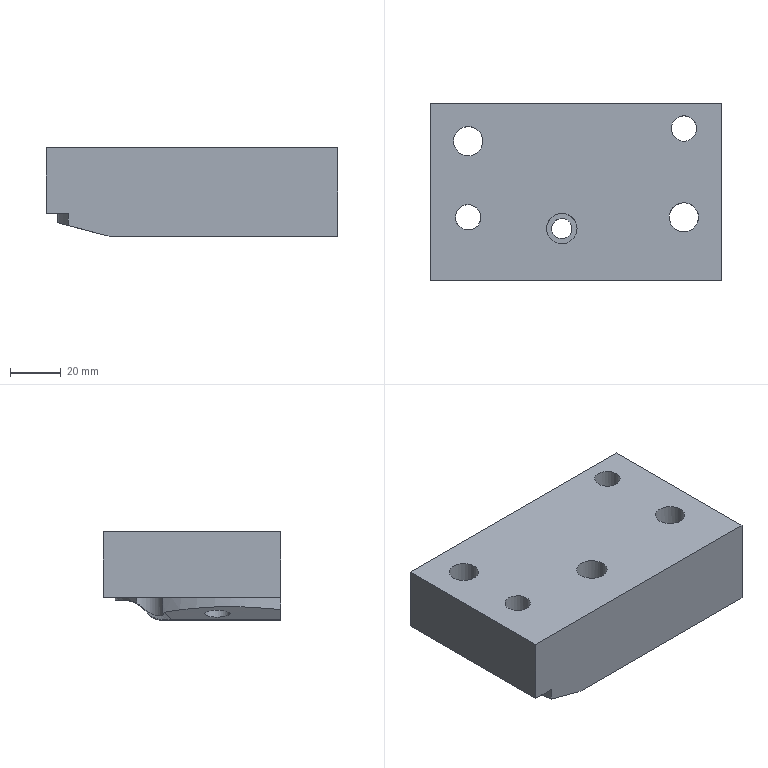Part | NX | features solid 2 | 1 solid | 30 faces | box 115 x 70 x 35 mm | volume 232873 mm3 | spline 16 | cylinder 7 | plane 7 | commonest cylinder face diameters 10 x2 11.5 x2 17.5 x2 8 x1